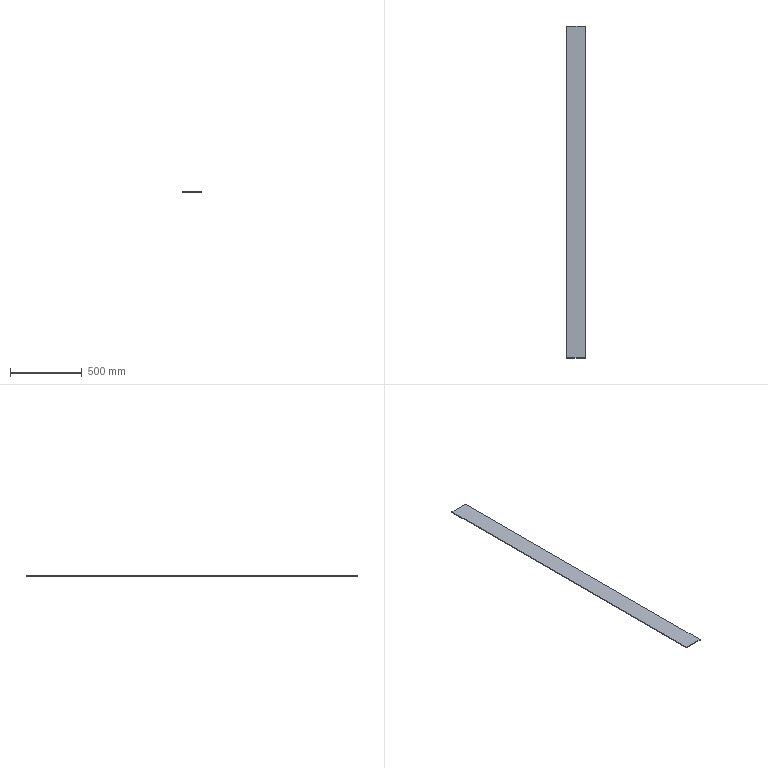Part | SolidWorks | features Extrusion 1, HoleWzd 1 | 1 solid | 6 faces | box 131 x 2310 x 5 mm | volume 1513050 mm3 | plane 6
STEP:
#1=CARTESIAN_POINT('',(65.5,-1155.,0.));
#2=VERTEX_POINT('',#1);
#3=CARTESIAN_POINT('',(65.5,1155.,0.));
#4=VERTEX_POINT('',#3);
#5=CARTESIAN_POINT('',(65.5,1155.,0.));
#6=DIRECTION('',(0.,1.,0.));
#7=VECTOR('',#6,1000.);
#8=LINE('',#5,#7);
#9=EDGE_CURVE('',#2,#4,#8,.T.);
#10=ORIENTED_EDGE('',*,*,#9,.T.);
#11=CARTESIAN_POINT('',(65.5,1155.,5.));
#12=VERTEX_POINT('',#11);
#13=CARTESIAN_POINT('',(65.5,1155.,5.));
#14=DIRECTION('',(0.,0.,-1.));
#15=VECTOR('',#14,1000.);
#16=LINE('',#13,#15);
#17=EDGE_CURVE('',#12,#4,#16,.T.);
#18=ORIENTED_EDGE('',*,*,#17,.F.);
#19=CARTESIAN_POINT('',(65.5,-1155.,5.));
#20=VERTEX_POINT('',#19);
#21=CARTESIAN_POINT('',(65.5,1155.,5.));
#22=DIRECTION('',(0.,1.,0.));
#23=VECTOR('',#22,1000.);
#24=LINE('',#21,#23);
#25=EDGE_CURVE('',#20,#12,#24,.T.);
#26=ORIENTED_EDGE('',*,*,#25,.F.);
#27=CARTESIAN_POINT('',(65.5,-1155.,5.));
#28=DIRECTION('',(0.,0.,-1.));
#29=VECTOR('',#28,1000.);
#30=LINE('',#27,#29);
#31=EDGE_CURVE('',#20,#2,#30,.T.);
#32=ORIENTED_EDGE('',*,*,#31,.T.);
#33=EDGE_LOOP('',(#10,#18,#26,#32));
#34=FACE_OUTER_BOUND('',#33,.T.);
#35=CARTESIAN_POINT('',(65.5,1155.,5.));
#36=DIRECTION('',(-1.,0.,0.));
#37=DIRECTION('',(0.,-1.,0.));
#38=AXIS2_PLACEMENT_3D('',#35,#36,#37);
#39=PLANE('',#38);
#40=ADVANCED_FACE('',(#34),#39,.F.);
#41=CARTESIAN_POINT('',(-65.5,1155.,0.));
#42=VERTEX_POINT('',#41);
#43=CARTESIAN_POINT('',(-65.5,1155.,0.));
#44=DIRECTION('',(-1.,0.,0.));
#45=VECTOR('',#44,1000.);
#46=LINE('',#43,#45);
#47=EDGE_CURVE('',#4,#42,#46,.T.);
#48=ORIENTED_EDGE('',*,*,#47,.T.);
#49=CARTESIAN_POINT('',(-65.5,1155.,5.));
#50=VERTEX_POINT('',#49);
#51=CARTESIAN_POINT('',(-65.5,1155.,5.));
#52=DIRECTION('',(0.,0.,-1.));
#53=VECTOR('',#52,1000.);
#54=LINE('',#51,#53);
#55=EDGE_CURVE('',#50,#42,#54,.T.);
#56=ORIENTED_EDGE('',*,*,#55,.F.);
#57=CARTESIAN_POINT('',(-65.5,1155.,5.));
#58=DIRECTION('',(-1.,0.,0.));
#59=VECTOR('',#58,1000.);
#60=LINE('',#57,#59);
#61=EDGE_CURVE('',#12,#50,#60,.T.);
#62=ORIENTED_EDGE('',*,*,#61,.F.);
#63=ORIENTED_EDGE('',*,*,#17,.T.);
#64=EDGE_LOOP('',(#48,#56,#62,#63));
#65=FACE_OUTER_BOUND('',#64,.T.);
#66=CARTESIAN_POINT('',(-65.5,1155.,5.));
#67=DIRECTION('',(0.,-1.,0.));
#68=DIRECTION('',(0.,0.,-1.));
#69=AXIS2_PLACEMENT_3D('',#66,#67,#68);
#70=PLANE('',#69);
#71=ADVANCED_FACE('',(#65),#70,.F.);
#72=CARTESIAN_POINT('',(-65.5,-1155.,0.));
#73=VERTEX_POINT('',#72);
#74=CARTESIAN_POINT('',(-65.5,1155.,0.));
#75=DIRECTION('',(0.,-1.,0.));
#76=VECTOR('',#75,1000.);
#77=LINE('',#74,#76);
#78=EDGE_CURVE('',#42,#73,#77,.T.);
#79=ORIENTED_EDGE('',*,*,#78,.T.);
#80=CARTESIAN_POINT('',(-65.5,-1155.,5.));
#81=VERTEX_POINT('',#80);
#82=CARTESIAN_POINT('',(-65.5,-1155.,5.));
#83=DIRECTION('',(0.,0.,-1.));
#84=VECTOR('',#83,1000.);
#85=LINE('',#82,#84);
#86=EDGE_CURVE('',#81,#73,#85,.T.);
#87=ORIENTED_EDGE('',*,*,#86,.F.);
#88=CARTESIAN_POINT('',(-65.5,1155.,5.));
#89=DIRECTION('',(0.,-1.,0.));
#90=VECTOR('',#89,1000.);
#91=LINE('',#88,#90);
#92=EDGE_CURVE('',#50,#81,#91,.T.);
#93=ORIENTED_EDGE('',*,*,#92,.F.);
#94=ORIENTED_EDGE('',*,*,#55,.T.);
#95=EDGE_LOOP('',(#79,#87,#93,#94));
#96=FACE_OUTER_BOUND('',#95,.T.);
#97=CARTESIAN_POINT('',(-65.5,1155.,5.));
#98=DIRECTION('',(1.,0.,0.));
#99=DIRECTION('',(0.,1.,0.));
#100=AXIS2_PLACEMENT_3D('',#97,#98,#99);
#101=PLANE('',#100);
#102=ADVANCED_FACE('',(#96),#101,.F.);
#103=CARTESIAN_POINT('',(-65.5,-1155.,0.));
#104=DIRECTION('',(1.,0.,0.));
#105=VECTOR('',#104,1000.);
#106=LINE('',#103,#105);
#107=EDGE_CURVE('',#73,#2,#106,.T.);
#108=ORIENTED_EDGE('',*,*,#107,.T.);
#109=ORIENTED_EDGE('',*,*,#31,.F.);
#110=CARTESIAN_POINT('',(-65.5,-1155.,5.));
#111=DIRECTION('',(1.,0.,0.));
#112=VECTOR('',#111,1000.);
#113=LINE('',#110,#112);
#114=EDGE_CURVE('',#81,#20,#113,.T.);
#115=ORIENTED_EDGE('',*,*,#114,.F.);
#116=ORIENTED_EDGE('',*,*,#86,.T.);
#117=EDGE_LOOP('',(#108,#109,#115,#116));
#118=FACE_OUTER_BOUND('',#117,.T.);
#119=CARTESIAN_POINT('',(-65.5,-1155.,5.));
#120=DIRECTION('',(0.,1.,0.));
#121=DIRECTION('',(0.,0.,1.));
#122=AXIS2_PLACEMENT_3D('',#119,#120,#121);
#123=PLANE('',#122);
#124=ADVANCED_FACE('',(#118),#123,.F.);
#125=ORIENTED_EDGE('',*,*,#25,.T.);
#126=ORIENTED_EDGE('',*,*,#61,.T.);
#127=ORIENTED_EDGE('',*,*,#92,.T.);
#128=ORIENTED_EDGE('',*,*,#114,.T.);
#129=EDGE_LOOP('',(#125,#126,#127,#128));
#130=FACE_OUTER_BOUND('',#129,.T.);
#131=CARTESIAN_POINT('',(0.,0.,5.));
#132=DIRECTION('',(0.,0.,1.));
#133=DIRECTION('',(1.,0.,0.));
#134=AXIS2_PLACEMENT_3D('',#131,#132,#133);
#135=PLANE('',#134);
#136=ADVANCED_FACE('',(#130),#135,.T.);
#137=ORIENTED_EDGE('',*,*,#9,.F.);
#138=ORIENTED_EDGE('',*,*,#107,.F.);
#139=ORIENTED_EDGE('',*,*,#78,.F.);
#140=ORIENTED_EDGE('',*,*,#47,.F.);
#141=EDGE_LOOP('',(#137,#138,#139,#140));
#142=FACE_OUTER_BOUND('',#141,.T.);
#143=CARTESIAN_POINT('',(0.,0.,0.));
#144=DIRECTION('',(0.,0.,1.));
#145=DIRECTION('',(1.,0.,0.));
#146=AXIS2_PLACEMENT_3D('',#143,#144,#145);
#147=PLANE('',#146);
#148=ADVANCED_FACE('',(#142),#147,.F.);
#149=CLOSED_SHELL('',(#40,#71,#102,#124,#136,#148));
#150=MANIFOLD_SOLID_BREP('',#149);
#151=CARTESIAN_POINT('',(0.,0.,0.));
#152=DIRECTION('',(0.,0.,1.));
#153=DIRECTION('',(1.,0.,0.));
#154=AXIS2_PLACEMENT_3D('',#151,#152,#153);
#155=(LENGTH_UNIT()NAMED_UNIT(*)SI_UNIT(.MILLI.,.METRE.));
#156=UNCERTAINTY_MEASURE_WITH_UNIT(LENGTH_MEASURE(0.00001),#155,'','');
#157=(NAMED_UNIT(*)PLANE_ANGLE_UNIT()SI_UNIT($,.RADIAN.));
#158=(NAMED_UNIT(*)SI_UNIT($,.STERADIAN.)SOLID_ANGLE_UNIT());
#159=(GEOMETRIC_REPRESENTATION_CONTEXT(3)GLOBAL_UNCERTAINTY_ASSIGNED_CONTEXT((#156))GLOBAL_UNIT_ASSIGNED_CONTEXT((#155,#157,#158))REPRESENTATION_CONTEXT('',''));
#160=ADVANCED_BREP_SHAPE_REPRESENTATION('',(#150,#154),#159);